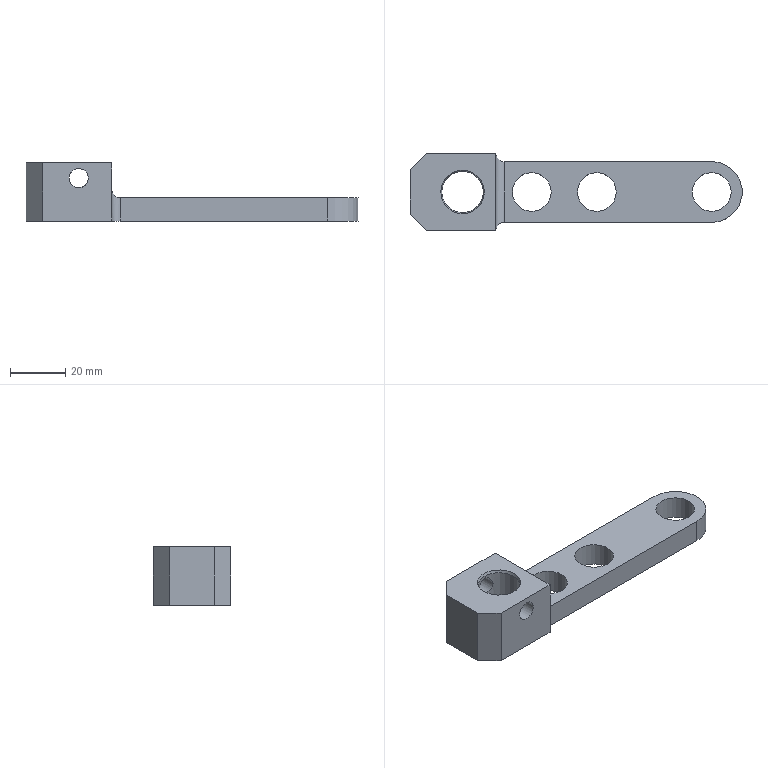Part | NX | 1 solid | 23 faces | box 120 x 28 x 21 mm | volume 25583 mm3 | plane 11 | cylinder 10 | cone 2 | commonest cylinder face diameters 6 x3 14 x3 7 x2 15 x1 22 x1
STEP:
#1=CARTESIAN_POINT('',(26.864,14.,21.));
#2=VERTEX_POINT('',#1);
#3=CARTESIAN_POINT('',(19.,14.,21.));
#4=DIRECTION('',(0.,0.,1.));
#5=DIRECTION('',(1.,0.,0.));
#6=AXIS2_PLACEMENT_3D('',#3,#4,#5);
#7=CIRCLE('',#6,7.864);
#8=EDGE_CURVE('',#2,#2,#7,.F.);
#9=ORIENTED_EDGE('',*,*,#8,.T.);
#10=EDGE_LOOP('',(#9));
#11=FACE_BOUND('',#10,.T.);
#12=CARTESIAN_POINT('',(6.,28.,21.));
#13=VERTEX_POINT('',#12);
#14=CARTESIAN_POINT('',(31.,28.,21.));
#15=VERTEX_POINT('',#14);
#16=CARTESIAN_POINT('',(60.,28.,21.));
#17=DIRECTION('',(1.,0.,0.));
#18=VECTOR('',#17,1000.);
#19=LINE('',#16,#18);
#20=EDGE_CURVE('',#13,#15,#19,.T.);
#21=ORIENTED_EDGE('',*,*,#20,.F.);
#22=CARTESIAN_POINT('',(0.,22.,21.));
#23=VERTEX_POINT('',#22);
#24=CARTESIAN_POINT('',(26.,48.,21.));
#25=DIRECTION('',(0.7071,0.7071,0.));
#26=VECTOR('',#25,1000.);
#27=LINE('',#24,#26);
#28=EDGE_CURVE('',#13,#23,#27,.F.);
#29=ORIENTED_EDGE('',*,*,#28,.T.);
#30=CARTESIAN_POINT('',(0.,6.,21.));
#31=VERTEX_POINT('',#30);
#32=CARTESIAN_POINT('',(0.,14.,21.));
#33=DIRECTION('',(0.,1.,0.));
#34=VECTOR('',#33,1000.);
#35=LINE('',#32,#34);
#36=EDGE_CURVE('',#31,#23,#35,.T.);
#37=ORIENTED_EDGE('',*,*,#36,.F.);
#38=CARTESIAN_POINT('',(6.,0.,21.));
#39=VERTEX_POINT('',#38);
#40=CARTESIAN_POINT('',(26.,-20.,21.));
#41=DIRECTION('',(-0.7071,0.7071,0.));
#42=VECTOR('',#41,1000.);
#43=LINE('',#40,#42);
#44=EDGE_CURVE('',#31,#39,#43,.F.);
#45=ORIENTED_EDGE('',*,*,#44,.T.);
#46=CARTESIAN_POINT('',(31.,0.,21.));
#47=VERTEX_POINT('',#46);
#48=CARTESIAN_POINT('',(60.,0.,21.));
#49=DIRECTION('',(-1.,0.,0.));
#50=VECTOR('',#49,1000.);
#51=LINE('',#48,#50);
#52=EDGE_CURVE('',#47,#39,#51,.T.);
#53=ORIENTED_EDGE('',*,*,#52,.F.);
#54=CARTESIAN_POINT('',(31.,14.,21.));
#55=DIRECTION('',(0.,-1.,0.));
#56=VECTOR('',#55,1000.);
#57=LINE('',#54,#56);
#58=EDGE_CURVE('',#15,#47,#57,.T.);
#59=ORIENTED_EDGE('',*,*,#58,.F.);
#60=EDGE_LOOP('',(#21,#29,#37,#45,#53,#59));
#61=FACE_BOUND('',#60,.T.);
#62=CARTESIAN_POINT('',(60.,14.,21.));
#63=DIRECTION('',(0.,0.,1.));
#64=DIRECTION('',(1.,0.,0.));
#65=AXIS2_PLACEMENT_3D('',#62,#63,#64);
#66=PLANE('',#65);
#67=ADVANCED_FACE('',(#11,#61),#66,.T.);
#68=CARTESIAN_POINT('',(31.,0.,11.5));
#69=VERTEX_POINT('',#68);
#70=CARTESIAN_POINT('',(31.,0.,0.));
#71=DIRECTION('',(0.,0.,-1.));
#72=VECTOR('',#71,1000.);
#73=LINE('',#70,#72);
#74=EDGE_CURVE('',#47,#69,#73,.T.);
#75=ORIENTED_EDGE('',*,*,#74,.T.);
#76=CARTESIAN_POINT('',(31.,28.,11.5));
#77=VERTEX_POINT('',#76);
#78=CARTESIAN_POINT('',(31.,25.,11.5));
#79=DIRECTION('',(0.,1.,0.));
#80=VECTOR('',#79,1000.);
#81=LINE('',#78,#80);
#82=EDGE_CURVE('',#69,#77,#81,.T.);
#83=ORIENTED_EDGE('',*,*,#82,.T.);
#84=CARTESIAN_POINT('',(31.,28.,0.));
#85=DIRECTION('',(0.,0.,1.));
#86=VECTOR('',#85,1000.);
#87=LINE('',#84,#86);
#88=EDGE_CURVE('',#15,#77,#87,.F.);
#89=ORIENTED_EDGE('',*,*,#88,.F.);
#90=ORIENTED_EDGE('',*,*,#58,.T.);
#91=EDGE_LOOP('',(#75,#83,#89,#90));
#92=FACE_BOUND('',#91,.T.);
#93=CARTESIAN_POINT('',(31.,14.,10.5));
#94=DIRECTION('',(-1.,0.,0.));
#95=DIRECTION('',(0.,0.,1.));
#96=AXIS2_PLACEMENT_3D('',#93,#94,#95);
#97=PLANE('',#96);
#98=ADVANCED_FACE('',(#92),#97,.F.);
#99=CARTESIAN_POINT('',(19.008,0.,12.));
#100=VERTEX_POINT('',#99);
#101=CARTESIAN_POINT('',(19.008,0.,15.5));
#102=DIRECTION('',(0.,-1.,0.));
#103=DIRECTION('',(0.,0.,-1.));
#104=AXIS2_PLACEMENT_3D('',#101,#102,#103);
#105=CIRCLE('',#104,3.5);
#106=EDGE_CURVE('',#100,#100,#105,.T.);
#107=ORIENTED_EDGE('',*,*,#106,.F.);
#108=EDGE_LOOP('',(#107));
#109=FACE_BOUND('',#108,.T.);
#110=ORIENTED_EDGE('',*,*,#52,.T.);
#111=CARTESIAN_POINT('',(6.,0.,0.));
#112=VERTEX_POINT('',#111);
#113=CARTESIAN_POINT('',(6.,0.,0.));
#114=DIRECTION('',(0.,0.,-1.));
#115=VECTOR('',#114,1000.);
#116=LINE('',#113,#115);
#117=EDGE_CURVE('',#39,#112,#116,.T.);
#118=ORIENTED_EDGE('',*,*,#117,.T.);
#119=CARTESIAN_POINT('',(31.,0.,0.));
#120=VERTEX_POINT('',#119);
#121=CARTESIAN_POINT('',(60.,0.,0.));
#122=DIRECTION('',(1.,0.,0.));
#123=VECTOR('',#122,1000.);
#124=LINE('',#121,#123);
#125=EDGE_CURVE('',#112,#120,#124,.T.);
#126=ORIENTED_EDGE('',*,*,#125,.T.);
#127=CARTESIAN_POINT('',(31.,0.,0.));
#128=DIRECTION('',(0.,0.,-1.));
#129=VECTOR('',#128,1000.);
#130=LINE('',#127,#129);
#131=EDGE_CURVE('',#69,#120,#130,.T.);
#132=ORIENTED_EDGE('',*,*,#131,.F.);
#133=ORIENTED_EDGE('',*,*,#74,.F.);
#134=EDGE_LOOP('',(#110,#118,#126,#132,#133));
#135=FACE_BOUND('',#134,.T.);
#136=CARTESIAN_POINT('',(60.,0.,0.));
#137=DIRECTION('',(0.,-1.,0.));
#138=DIRECTION('',(0.,0.,-1.));
#139=AXIS2_PLACEMENT_3D('',#136,#137,#138);
#140=PLANE('',#139);
#141=ADVANCED_FACE('',(#109,#135),#140,.T.);
#142=ORIENTED_EDGE('',*,*,#36,.T.);
#143=CARTESIAN_POINT('',(0.,22.,0.));
#144=VERTEX_POINT('',#143);
#145=CARTESIAN_POINT('',(0.,22.,0.));
#146=DIRECTION('',(0.,0.,-1.));
#147=VECTOR('',#146,1000.);
#148=LINE('',#145,#147);
#149=EDGE_CURVE('',#23,#144,#148,.T.);
#150=ORIENTED_EDGE('',*,*,#149,.T.);
#151=CARTESIAN_POINT('',(0.,6.,0.));
#152=VERTEX_POINT('',#151);
#153=CARTESIAN_POINT('',(0.,14.,0.));
#154=DIRECTION('',(0.,-1.,0.));
#155=VECTOR('',#154,1000.);
#156=LINE('',#153,#155);
#157=EDGE_CURVE('',#144,#152,#156,.T.);
#158=ORIENTED_EDGE('',*,*,#157,.T.);
#159=CARTESIAN_POINT('',(0.,6.,0.));
#160=DIRECTION('',(0.,0.,1.));
#161=VECTOR('',#160,1000.);
#162=LINE('',#159,#161);
#163=EDGE_CURVE('',#152,#31,#162,.T.);
#164=ORIENTED_EDGE('',*,*,#163,.T.);
#165=EDGE_LOOP('',(#142,#150,#158,#164));
#166=FACE_BOUND('',#165,.T.);
#167=CARTESIAN_POINT('',(0.,14.,0.));
#168=DIRECTION('',(-1.,0.,0.));
#169=DIRECTION('',(0.,0.,1.));
#170=AXIS2_PLACEMENT_3D('',#167,#168,#169);
#171=PLANE('',#170);
#172=ADVANCED_FACE('',(#166),#171,.T.);
#173=CARTESIAN_POINT('',(19.008,28.,12.));
#174=VERTEX_POINT('',#173);
#175=CARTESIAN_POINT('',(19.008,28.,15.5));
#176=DIRECTION('',(0.,-1.,0.));
#177=DIRECTION('',(0.,0.,-1.));
#178=AXIS2_PLACEMENT_3D('',#175,#176,#177);
#179=CIRCLE('',#178,3.5);
#180=EDGE_CURVE('',#174,#174,#179,.T.);
#181=ORIENTED_EDGE('',*,*,#180,.T.);
#182=EDGE_LOOP('',(#181));
#183=FACE_BOUND('',#182,.T.);
#184=CARTESIAN_POINT('',(31.,28.,0.));
#185=VERTEX_POINT('',#184);
#186=CARTESIAN_POINT('',(6.,28.,0.));
#187=VERTEX_POINT('',#186);
#188=CARTESIAN_POINT('',(60.,28.,0.));
#189=DIRECTION('',(-1.,0.,0.));
#190=VECTOR('',#189,1000.);
#191=LINE('',#188,#190);
#192=EDGE_CURVE('',#185,#187,#191,.T.);
#193=ORIENTED_EDGE('',*,*,#192,.T.);
#194=CARTESIAN_POINT('',(6.,28.,0.));
#195=DIRECTION('',(0.,0.,1.));
#196=VECTOR('',#195,1000.);
#197=LINE('',#194,#196);
#198=EDGE_CURVE('',#187,#13,#197,.T.);
#199=ORIENTED_EDGE('',*,*,#198,.T.);
#200=ORIENTED_EDGE('',*,*,#20,.T.);
#201=ORIENTED_EDGE('',*,*,#88,.T.);
#202=CARTESIAN_POINT('',(31.,28.,0.));
#203=DIRECTION('',(0.,0.,1.));
#204=VECTOR('',#203,1000.);
#205=LINE('',#202,#204);
#206=EDGE_CURVE('',#77,#185,#205,.F.);
#207=ORIENTED_EDGE('',*,*,#206,.T.);
#208=EDGE_LOOP('',(#193,#199,#200,#201,#207));
#209=FACE_BOUND('',#208,.T.);
#210=CARTESIAN_POINT('',(60.,28.,0.));
#211=DIRECTION('',(0.,1.,0.));
#212=DIRECTION('',(0.,0.,1.));
#213=AXIS2_PLACEMENT_3D('',#210,#211,#212);
#214=PLANE('',#213);
#215=ADVANCED_FACE('',(#183,#209),#214,.T.);
#216=CARTESIAN_POINT('',(11.136,14.,0.));
#217=VERTEX_POINT('',#216);
#218=CARTESIAN_POINT('',(19.,14.,0.));
#219=DIRECTION('',(0.,0.,-1.));
#220=DIRECTION('',(-1.,0.,0.));
#221=AXIS2_PLACEMENT_3D('',#218,#219,#220);
#222=CIRCLE('',#221,7.864);
#223=EDGE_CURVE('',#217,#217,#222,.F.);
#224=ORIENTED_EDGE('',*,*,#223,.T.);
#225=EDGE_LOOP('',(#224));
#226=FACE_BOUND('',#225,.T.);
#227=CARTESIAN_POINT('',(102.,14.,0.));
#228=VERTEX_POINT('',#227);
#229=CARTESIAN_POINT('',(109.,14.,0.));
#230=DIRECTION('',(0.,0.,-1.));
#231=DIRECTION('',(-1.,0.,0.));
#232=AXIS2_PLACEMENT_3D('',#229,#230,#231);
#233=CIRCLE('',#232,7.);
#234=EDGE_CURVE('',#228,#228,#233,.T.);
#235=ORIENTED_EDGE('',*,*,#234,.F.);
#236=EDGE_LOOP('',(#235));
#237=FACE_BOUND('',#236,.T.);
#238=CARTESIAN_POINT('',(60.5,14.,0.));
#239=VERTEX_POINT('',#238);
#240=CARTESIAN_POINT('',(67.5,14.,0.));
#241=DIRECTION('',(0.,0.,-1.));
#242=DIRECTION('',(-1.,0.,0.));
#243=AXIS2_PLACEMENT_3D('',#240,#241,#242);
#244=CIRCLE('',#243,7.);
#245=EDGE_CURVE('',#239,#239,#244,.T.);
#246=ORIENTED_EDGE('',*,*,#245,.F.);
#247=EDGE_LOOP('',(#246));
#248=FACE_BOUND('',#247,.T.);
#249=CARTESIAN_POINT('',(37.,14.,0.));
#250=VERTEX_POINT('',#249);
#251=CARTESIAN_POINT('',(44.,14.,0.));
#252=DIRECTION('',(0.,0.,-1.));
#253=DIRECTION('',(-1.,0.,0.));
#254=AXIS2_PLACEMENT_3D('',#251,#252,#253);
#255=CIRCLE('',#254,7.);
#256=EDGE_CURVE('',#250,#250,#255,.T.);
#257=ORIENTED_EDGE('',*,*,#256,.F.);
#258=EDGE_LOOP('',(#257));
#259=FACE_BOUND('',#258,.T.);
#260=ORIENTED_EDGE('',*,*,#157,.F.);
#261=CARTESIAN_POINT('',(26.,48.,0.));
#262=DIRECTION('',(-0.7071,-0.7071,0.));
#263=VECTOR('',#262,1000.);
#264=LINE('',#261,#263);
#265=EDGE_CURVE('',#144,#187,#264,.F.);
#266=ORIENTED_EDGE('',*,*,#265,.T.);
#267=ORIENTED_EDGE('',*,*,#192,.F.);
#268=CARTESIAN_POINT('',(34.,25.,0.));
#269=VERTEX_POINT('',#268);
#270=CARTESIAN_POINT('',(34.,28.,0.));
#271=DIRECTION('',(0.,0.,-1.));
#272=DIRECTION('',(-1.,0.,0.));
#273=AXIS2_PLACEMENT_3D('',#270,#271,#272);
#274=CIRCLE('',#273,3.);
#275=EDGE_CURVE('',#185,#269,#274,.F.);
#276=ORIENTED_EDGE('',*,*,#275,.T.);
#277=CARTESIAN_POINT('',(109.,25.,0.));
#278=VERTEX_POINT('',#277);
#279=CARTESIAN_POINT('',(60.,25.,0.));
#280=DIRECTION('',(-1.,0.,0.));
#281=VECTOR('',#280,1000.);
#282=LINE('',#279,#281);
#283=EDGE_CURVE('',#278,#269,#282,.T.);
#284=ORIENTED_EDGE('',*,*,#283,.F.);
#285=CARTESIAN_POINT('',(109.,3.,0.));
#286=VERTEX_POINT('',#285);
#287=CARTESIAN_POINT('',(109.,14.,0.));
#288=DIRECTION('',(0.,0.,-1.));
#289=DIRECTION('',(-1.,0.,0.));
#290=AXIS2_PLACEMENT_3D('',#287,#288,#289);
#291=CIRCLE('',#290,11.);
#292=EDGE_CURVE('',#278,#286,#291,.T.);
#293=ORIENTED_EDGE('',*,*,#292,.T.);
#294=CARTESIAN_POINT('',(34.,3.,0.));
#295=VERTEX_POINT('',#294);
#296=CARTESIAN_POINT('',(60.,3.,0.));
#297=DIRECTION('',(1.,0.,0.));
#298=VECTOR('',#297,1000.);
#299=LINE('',#296,#298);
#300=EDGE_CURVE('',#295,#286,#299,.T.);
#301=ORIENTED_EDGE('',*,*,#300,.F.);
#302=CARTESIAN_POINT('',(34.,0.,0.));
#303=DIRECTION('',(0.,0.,-1.));
#304=DIRECTION('',(-1.,0.,0.));
#305=AXIS2_PLACEMENT_3D('',#302,#303,#304);
#306=CIRCLE('',#305,3.);
#307=EDGE_CURVE('',#295,#120,#306,.F.);
#308=ORIENTED_EDGE('',*,*,#307,.T.);
#309=ORIENTED_EDGE('',*,*,#125,.F.);
#310=CARTESIAN_POINT('',(26.,-20.,0.));
#311=DIRECTION('',(0.7071,-0.7071,0.));
#312=VECTOR('',#311,1000.);
#313=LINE('',#310,#312);
#314=EDGE_CURVE('',#112,#152,#313,.F.);
#315=ORIENTED_EDGE('',*,*,#314,.T.);
#316=EDGE_LOOP('',(#260,#266,#267,#276,#284,#293,#301,#308,#309,#315));
#317=FACE_BOUND('',#316,.T.);
#318=CARTESIAN_POINT('',(60.,14.,0.));
#319=DIRECTION('',(0.,0.,-1.));
#320=DIRECTION('',(-1.,0.,0.));
#321=AXIS2_PLACEMENT_3D('',#318,#319,#320);
#322=PLANE('',#321);
#323=ADVANCED_FACE('',(#226,#237,#248,#259,#317),#322,.T.);
#324=ORIENTED_EDGE('',*,*,#265,.F.);
#325=ORIENTED_EDGE('',*,*,#149,.F.);
#326=ORIENTED_EDGE('',*,*,#28,.F.);
#327=ORIENTED_EDGE('',*,*,#198,.F.);
#328=EDGE_LOOP('',(#324,#325,#326,#327));
#329=FACE_BOUND('',#328,.T.);
#330=CARTESIAN_POINT('',(6.,28.,0.));
#331=DIRECTION('',(0.7071,-0.7071,0.));
#332=DIRECTION('',(0.,0.,1.));
#333=AXIS2_PLACEMENT_3D('',#330,#331,#332);
#334=PLANE('',#333);
#335=ADVANCED_FACE('',(#329),#334,.F.);
#336=ORIENTED_EDGE('',*,*,#314,.F.);
#337=ORIENTED_EDGE('',*,*,#117,.F.);
#338=ORIENTED_EDGE('',*,*,#44,.F.);
#339=ORIENTED_EDGE('',*,*,#163,.F.);
#340=EDGE_LOOP('',(#336,#337,#338,#339));
#341=FACE_BOUND('',#340,.T.);
#342=CARTESIAN_POINT('',(0.,6.,0.));
#343=DIRECTION('',(0.7071,0.7071,0.));
#344=DIRECTION('',(0.,0.,1.));
#345=AXIS2_PLACEMENT_3D('',#342,#343,#344);
#346=PLANE('',#345);
#347=ADVANCED_FACE('',(#341),#346,.F.);
#348=ORIENTED_EDGE('',*,*,#283,.T.);
#349=CARTESIAN_POINT('',(34.,25.,8.5));
#350=VERTEX_POINT('',#349);
#351=CARTESIAN_POINT('',(34.,25.,0.));
#352=DIRECTION('',(0.,0.,-1.));
#353=VECTOR('',#352,1000.);
#354=LINE('',#351,#353);
#355=EDGE_CURVE('',#269,#350,#354,.F.);
#356=ORIENTED_EDGE('',*,*,#355,.T.);
#357=CARTESIAN_POINT('',(109.,25.,8.5));
#358=VERTEX_POINT('',#357);
#359=CARTESIAN_POINT('',(75.5,25.,8.5));
#360=DIRECTION('',(1.,0.,0.));
#361=VECTOR('',#360,1000.);
#362=LINE('',#359,#361);
#363=EDGE_CURVE('',#350,#358,#362,.T.);
#364=ORIENTED_EDGE('',*,*,#363,.T.);
#365=CARTESIAN_POINT('',(109.,25.,0.));
#366=DIRECTION('',(0.,0.,1.));
#367=VECTOR('',#366,1000.);
#368=LINE('',#365,#367);
#369=EDGE_CURVE('',#358,#278,#368,.F.);
#370=ORIENTED_EDGE('',*,*,#369,.T.);
#371=EDGE_LOOP('',(#348,#356,#364,#370));
#372=FACE_BOUND('',#371,.T.);
#373=CARTESIAN_POINT('',(60.,25.,0.));
#374=DIRECTION('',(0.,1.,0.));
#375=DIRECTION('',(0.,0.,1.));
#376=AXIS2_PLACEMENT_3D('',#373,#374,#375);
#377=PLANE('',#376);
#378=ADVANCED_FACE('',(#372),#377,.T.);
#379=CARTESIAN_POINT('',(34.,3.,8.5));
#380=VERTEX_POINT('',#379);
#381=CARTESIAN_POINT('',(109.,3.,8.5));
#382=VERTEX_POINT('',#381);
#383=CARTESIAN_POINT('',(60.,3.,8.5));
#384=DIRECTION('',(1.,0.,0.));
#385=VECTOR('',#384,1000.);
#386=LINE('',#383,#385);
#387=EDGE_CURVE('',#380,#382,#386,.T.);
#388=ORIENTED_EDGE('',*,*,#387,.F.);
#389=CARTESIAN_POINT('',(34.,3.,0.));
#390=DIRECTION('',(0.,0.,1.));
#391=VECTOR('',#390,1000.);
#392=LINE('',#389,#391);
#393=EDGE_CURVE('',#380,#295,#392,.F.);
#394=ORIENTED_EDGE('',*,*,#393,.T.);
#395=ORIENTED_EDGE('',*,*,#300,.T.);
#396=CARTESIAN_POINT('',(109.,3.,0.));
#397=DIRECTION('',(0.,0.,1.));
#398=VECTOR('',#397,1000.);
#399=LINE('',#396,#398);
#400=EDGE_CURVE('',#286,#382,#399,.T.);
#401=ORIENTED_EDGE('',*,*,#400,.T.);
#402=EDGE_LOOP('',(#388,#394,#395,#401));
#403=FACE_BOUND('',#402,.T.);
#404=CARTESIAN_POINT('',(60.,3.,0.));
#405=DIRECTION('',(0.,-1.,0.));
#406=DIRECTION('',(0.,0.,-1.));
#407=AXIS2_PLACEMENT_3D('',#404,#405,#406);
#408=PLANE('',#407);
#409=ADVANCED_FACE('',(#403),#408,.T.);
#410=CARTESIAN_POINT('',(102.,14.,8.5));
#411=VERTEX_POINT('',#410);
#412=CARTESIAN_POINT('',(109.,14.,8.5));
#413=DIRECTION('',(0.,0.,-1.));
#414=DIRECTION('',(-1.,0.,0.));
#415=AXIS2_PLACEMENT_3D('',#412,#413,#414);
#416=CIRCLE('',#415,7.);
#417=EDGE_CURVE('',#411,#411,#416,.T.);
#418=ORIENTED_EDGE('',*,*,#417,.T.);
#419=EDGE_LOOP('',(#418));
#420=FACE_BOUND('',#419,.T.);
#421=CARTESIAN_POINT('',(60.5,14.,8.5));
#422=VERTEX_POINT('',#421);
#423=CARTESIAN_POINT('',(67.5,14.,8.5));
#424=DIRECTION('',(0.,0.,-1.));
#425=DIRECTION('',(-1.,0.,0.));
#426=AXIS2_PLACEMENT_3D('',#423,#424,#425);
#427=CIRCLE('',#426,7.);
#428=EDGE_CURVE('',#422,#422,#427,.T.);
#429=ORIENTED_EDGE('',*,*,#428,.T.);
#430=EDGE_LOOP('',(#429));
#431=FACE_BOUND('',#430,.T.);
#432=CARTESIAN_POINT('',(37.,14.,8.5));
#433=VERTEX_POINT('',#432);
#434=CARTESIAN_POINT('',(44.,14.,8.5));
#435=DIRECTION('',(0.,0.,-1.));
#436=DIRECTION('',(-1.,0.,0.));
#437=AXIS2_PLACEMENT_3D('',#434,#435,#436);
#438=CIRCLE('',#437,7.);
#439=EDGE_CURVE('',#433,#433,#438,.T.);
#440=ORIENTED_EDGE('',*,*,#439,.T.);
#441=EDGE_LOOP('',(#440));
#442=FACE_BOUND('',#441,.T.);
#443=ORIENTED_EDGE('',*,*,#363,.F.);
#444=CARTESIAN_POINT('',(34.,3.,8.5));
#445=DIRECTION('',(0.,1.,0.));
#446=VECTOR('',#445,1000.);
#447=LINE('',#444,#446);
#448=EDGE_CURVE('',#350,#380,#447,.F.);
#449=ORIENTED_EDGE('',*,*,#448,.T.);
#450=ORIENTED_EDGE('',*,*,#387,.T.);
#451=CARTESIAN_POINT('',(109.,14.,8.5));
#452=DIRECTION('',(0.,0.,-1.));
#453=DIRECTION('',(-1.,0.,0.));
#454=AXIS2_PLACEMENT_3D('',#451,#452,#453);
#455=CIRCLE('',#454,11.);
#456=EDGE_CURVE('',#382,#358,#455,.F.);
#457=ORIENTED_EDGE('',*,*,#456,.T.);
#458=EDGE_LOOP('',(#443,#449,#450,#457));
#459=FACE_BOUND('',#458,.T.);
#460=CARTESIAN_POINT('',(75.5,14.,8.5));
#461=DIRECTION('',(0.,0.,-1.));
#462=DIRECTION('',(-1.,0.,0.));
#463=AXIS2_PLACEMENT_3D('',#460,#461,#462);
#464=PLANE('',#463);
#465=ADVANCED_FACE('',(#420,#431,#442,#459),#464,.F.);
#466=ORIENTED_EDGE('',*,*,#456,.F.);
#467=ORIENTED_EDGE('',*,*,#400,.F.);
#468=ORIENTED_EDGE('',*,*,#292,.F.);
#469=ORIENTED_EDGE('',*,*,#369,.F.);
#470=EDGE_LOOP('',(#466,#467,#468,#469));
#471=FACE_BOUND('',#470,.T.);
#472=CARTESIAN_POINT('',(109.,14.,0.));
#473=DIRECTION('',(0.,0.,1.));
#474=DIRECTION('',(1.,0.,0.));
#475=AXIS2_PLACEMENT_3D('',#472,#473,#474);
#476=CYLINDRICAL_SURFACE('',#475,11.);
#477=ADVANCED_FACE('',(#471),#476,.T.);
#478=ORIENTED_EDGE('',*,*,#307,.F.);
#479=ORIENTED_EDGE('',*,*,#393,.F.);
#480=CARTESIAN_POINT('',(34.,0.,11.5));
#481=DIRECTION('',(0.,-0.7071,-0.7071));
#482=DIRECTION('',(0.,-0.7071,0.7071));
#483=AXIS2_PLACEMENT_3D('',#480,#481,#482);
#484=ELLIPSE('',#483,4.243,3.);
#485=EDGE_CURVE('',#69,#380,#484,.T.);
#486=ORIENTED_EDGE('',*,*,#485,.F.);
#487=ORIENTED_EDGE('',*,*,#131,.T.);
#488=EDGE_LOOP('',(#478,#479,#486,#487));
#489=FACE_BOUND('',#488,.T.);
#490=CARTESIAN_POINT('',(34.,0.,10.5));
#491=DIRECTION('',(0.,0.,1.));
#492=DIRECTION('',(1.,0.,0.));
#493=AXIS2_PLACEMENT_3D('',#490,#491,#492);
#494=CYLINDRICAL_SURFACE('',#493,3.);
#495=ADVANCED_FACE('',(#489),#494,.F.);
#496=ORIENTED_EDGE('',*,*,#485,.T.);
#497=ORIENTED_EDGE('',*,*,#448,.F.);
#498=CARTESIAN_POINT('',(34.,28.,11.5));
#499=DIRECTION('',(0.,0.7071,-0.7071));
#500=DIRECTION('',(0.,-0.7071,-0.7071));
#501=AXIS2_PLACEMENT_3D('',#498,#499,#500);
#502=ELLIPSE('',#501,4.243,3.);
#503=EDGE_CURVE('',#77,#350,#502,.F.);
#504=ORIENTED_EDGE('',*,*,#503,.F.);
#505=ORIENTED_EDGE('',*,*,#82,.F.);
#506=EDGE_LOOP('',(#496,#497,#504,#505));
#507=FACE_BOUND('',#506,.T.);
#508=CARTESIAN_POINT('',(34.,14.,11.5));
#509=DIRECTION('',(0.,-1.,0.));
#510=DIRECTION('',(0.,0.,-1.));
#511=AXIS2_PLACEMENT_3D('',#508,#509,#510);
#512=CYLINDRICAL_SURFACE('',#511,3.);
#513=ADVANCED_FACE('',(#507),#512,.F.);
#514=ORIENTED_EDGE('',*,*,#275,.F.);
#515=ORIENTED_EDGE('',*,*,#206,.F.);
#516=ORIENTED_EDGE('',*,*,#503,.T.);
#517=ORIENTED_EDGE('',*,*,#355,.F.);
#518=EDGE_LOOP('',(#514,#515,#516,#517));
#519=FACE_BOUND('',#518,.T.);
#520=CARTESIAN_POINT('',(34.,28.,10.5));
#521=DIRECTION('',(0.,0.,-1.));
#522=DIRECTION('',(-1.,0.,0.));
#523=AXIS2_PLACEMENT_3D('',#520,#521,#522);
#524=CYLINDRICAL_SURFACE('',#523,3.);
#525=ADVANCED_FACE('',(#519),#524,.F.);
#526=ORIENTED_EDGE('',*,*,#256,.T.);
#527=EDGE_LOOP('',(#526));
#528=FACE_BOUND('',#527,.T.);
#529=ORIENTED_EDGE('',*,*,#439,.F.);
#530=EDGE_LOOP('',(#529));
#531=FACE_BOUND('',#530,.T.);
#532=CARTESIAN_POINT('',(44.,14.,12.5));
#533=DIRECTION('',(0.,0.,-1.));
#534=DIRECTION('',(-1.,0.,0.));
#535=AXIS2_PLACEMENT_3D('',#532,#533,#534);
#536=CYLINDRICAL_SURFACE('',#535,7.);
#537=ADVANCED_FACE('',(#528,#531),#536,.F.);
#538=ORIENTED_EDGE('',*,*,#245,.T.);
#539=EDGE_LOOP('',(#538));
#540=FACE_BOUND('',#539,.T.);
#541=ORIENTED_EDGE('',*,*,#428,.F.);
#542=EDGE_LOOP('',(#541));
#543=FACE_BOUND('',#542,.T.);
#544=CARTESIAN_POINT('',(67.5,14.,12.5));
#545=DIRECTION('',(0.,0.,-1.));
#546=DIRECTION('',(-1.,0.,0.));
#547=AXIS2_PLACEMENT_3D('',#544,#545,#546);
#548=CYLINDRICAL_SURFACE('',#547,7.);
#549=ADVANCED_FACE('',(#540,#543),#548,.F.);
#550=ORIENTED_EDGE('',*,*,#234,.T.);
#551=EDGE_LOOP('',(#550));
#552=FACE_BOUND('',#551,.T.);
#553=ORIENTED_EDGE('',*,*,#417,.F.);
#554=EDGE_LOOP('',(#553));
#555=FACE_BOUND('',#554,.T.);
#556=CARTESIAN_POINT('',(109.,14.,12.5));
#557=DIRECTION('',(0.,0.,-1.));
#558=DIRECTION('',(-1.,0.,0.));
#559=AXIS2_PLACEMENT_3D('',#556,#557,#558);
#560=CYLINDRICAL_SURFACE('',#559,7.);
#561=ADVANCED_FACE('',(#552,#555),#560,.F.);
#562=CARTESIAN_POINT('',(11.5,14.,1.));
#563=VERTEX_POINT('',#562);
#564=CARTESIAN_POINT('',(19.,14.,1.));
#565=DIRECTION('',(0.,0.,-1.));
#566=DIRECTION('',(-1.,0.,0.));
#567=AXIS2_PLACEMENT_3D('',#564,#565,#566);
#568=CIRCLE('',#567,7.5);
#569=EDGE_CURVE('',#563,#563,#568,.T.);
#570=ORIENTED_EDGE('',*,*,#569,.T.);
#571=EDGE_LOOP('',(#570));
#572=FACE_BOUND('',#571,.T.);
#573=CARTESIAN_POINT('',(26.5,14.,20.));
#574=VERTEX_POINT('',#573);
#575=CARTESIAN_POINT('',(19.,14.,20.));
#576=DIRECTION('',(0.,0.,1.));
#577=DIRECTION('',(1.,0.,0.));
#578=AXIS2_PLACEMENT_3D('',#575,#576,#577);
#579=CIRCLE('',#578,7.5);
#580=EDGE_CURVE('',#574,#574,#579,.T.);
#581=ORIENTED_EDGE('',*,*,#580,.T.);
#582=EDGE_LOOP('',(#581));
#583=FACE_BOUND('',#582,.T.);
#584=CARTESIAN_POINT('',(19.008,21.5,12.));
#585=VERTEX_POINT('',#584);
#586=CARTESIAN_POINT('',(21.755,21.089,12.76));
#587=CARTESIAN_POINT('',(19.007,21.704,11.619));
#588=CARTESIAN_POINT('',(16.263,21.095,12.762));
#589=CARTESIAN_POINT('',(15.13,20.409,15.491));
#590=CARTESIAN_POINT('',(16.263,21.094,18.241));
#591=CARTESIAN_POINT('',(18.999,21.704,19.38));
#592=CARTESIAN_POINT('',(21.753,21.09,18.241));
#593=CARTESIAN_POINT('',(22.885,20.399,15.508));
#594=CARTESIAN_POINT('',(21.755,21.089,12.76));
#595=CARTESIAN_POINT('',(19.007,21.704,11.619));
#596=CARTESIAN_POINT('',(16.263,21.095,12.762));
#597=B_SPLINE_CURVE_WITH_KNOTS('',3,(#586,#587,#588,#589,#590,#591,#592,#593,#594,#595,#596),.UNSPECIFIED.,.T.,.F.,(1,1,1,1,1,1,1,1,1,1,1,1,1,1,1),(-0.008324,-0.005549,-0.002775,0.,0.002775,0.005549,0.008324,0.0111,0.01387,0.01665,0.01942,0.0222,0.02497,0.02775,0.03052),.UNSPECIFIED.);
#598=EDGE_CURVE('',#585,#585,#597,.T.);
#599=ORIENTED_EDGE('',*,*,#598,.T.);
#600=EDGE_LOOP('',(#599));
#601=FACE_BOUND('',#600,.T.);
#602=CARTESIAN_POINT('',(19.008,6.5,12.));
#603=VERTEX_POINT('',#602);
#604=CARTESIAN_POINT('',(16.259,6.906,12.76));
#605=CARTESIAN_POINT('',(19.009,6.296,11.619));
#606=CARTESIAN_POINT('',(21.751,6.91,12.762));
#607=CARTESIAN_POINT('',(22.885,7.601,15.489));
#608=CARTESIAN_POINT('',(21.754,6.912,18.239));
#609=CARTESIAN_POINT('',(19.02,6.296,19.38));
#610=CARTESIAN_POINT('',(16.264,6.903,18.242));
#611=CARTESIAN_POINT('',(15.131,7.592,15.51));
#612=CARTESIAN_POINT('',(16.259,6.906,12.76));
#613=CARTESIAN_POINT('',(19.009,6.296,11.619));
#614=CARTESIAN_POINT('',(21.751,6.91,12.762));
#615=B_SPLINE_CURVE_WITH_KNOTS('',3,(#604,#605,#606,#607,#608,#609,#610,#611,#612,#613,#614),.UNSPECIFIED.,.T.,.F.,(1,1,1,1,1,1,1,1,1,1,1,1,1,1,1),(-0.008324,-0.005549,-0.002775,0.,0.002775,0.005549,0.008324,0.0111,0.01387,0.01665,0.01942,0.0222,0.02497,0.02775,0.03052),.UNSPECIFIED.);
#616=EDGE_CURVE('',#603,#603,#615,.T.);
#617=ORIENTED_EDGE('',*,*,#616,.T.);
#618=EDGE_LOOP('',(#617));
#619=FACE_BOUND('',#618,.T.);
#620=CARTESIAN_POINT('',(19.,14.,12.5));
#621=DIRECTION('',(0.,0.,-1.));
#622=DIRECTION('',(-1.,0.,0.));
#623=AXIS2_PLACEMENT_3D('',#620,#621,#622);
#624=CYLINDRICAL_SURFACE('',#623,7.5);
#625=ADVANCED_FACE('',(#572,#583,#601,#619),#624,.F.);
#626=ORIENTED_EDGE('',*,*,#106,.T.);
#627=EDGE_LOOP('',(#626));
#628=FACE_BOUND('',#627,.T.);
#629=ORIENTED_EDGE('',*,*,#616,.F.);
#630=EDGE_LOOP('',(#629));
#631=FACE_BOUND('',#630,.T.);
#632=CARTESIAN_POINT('',(19.008,28.,15.5));
#633=DIRECTION('',(0.,-1.,0.));
#634=DIRECTION('',(0.,0.,-1.));
#635=AXIS2_PLACEMENT_3D('',#632,#633,#634);
#636=CYLINDRICAL_SURFACE('',#635,3.5);
#637=ADVANCED_FACE('',(#628,#631),#636,.F.);
#638=ORIENTED_EDGE('',*,*,#180,.F.);
#639=EDGE_LOOP('',(#638));
#640=FACE_BOUND('',#639,.T.);
#641=ORIENTED_EDGE('',*,*,#598,.F.);
#642=EDGE_LOOP('',(#641));
#643=FACE_BOUND('',#642,.T.);
#644=CARTESIAN_POINT('',(19.008,28.,15.5));
#645=DIRECTION('',(0.,-1.,0.));
#646=DIRECTION('',(0.,0.,-1.));
#647=AXIS2_PLACEMENT_3D('',#644,#645,#646);
#648=CYLINDRICAL_SURFACE('',#647,3.5);
#649=ADVANCED_FACE('',(#640,#643),#648,.F.);
#650=ORIENTED_EDGE('',*,*,#223,.F.);
#651=EDGE_LOOP('',(#650));
#652=FACE_BOUND('',#651,.T.);
#653=ORIENTED_EDGE('',*,*,#569,.F.);
#654=EDGE_LOOP('',(#653));
#655=FACE_BOUND('',#654,.T.);
#656=CARTESIAN_POINT('',(19.,14.,1.));
#657=DIRECTION('',(0.,0.,-1.));
#658=DIRECTION('',(-1.,0.,0.));
#659=AXIS2_PLACEMENT_3D('',#656,#657,#658);
#660=CONICAL_SURFACE('',#659,7.5,0.3491);
#661=ADVANCED_FACE('',(#652,#655),#660,.F.);
#662=ORIENTED_EDGE('',*,*,#8,.F.);
#663=EDGE_LOOP('',(#662));
#664=FACE_BOUND('',#663,.T.);
#665=ORIENTED_EDGE('',*,*,#580,.F.);
#666=EDGE_LOOP('',(#665));
#667=FACE_BOUND('',#666,.T.);
#668=CARTESIAN_POINT('',(19.,14.,20.));
#669=DIRECTION('',(0.,0.,1.));
#670=DIRECTION('',(1.,0.,0.));
#671=AXIS2_PLACEMENT_3D('',#668,#669,#670);
#672=CONICAL_SURFACE('',#671,7.5,0.3491);
#673=ADVANCED_FACE('',(#664,#667),#672,.F.);
#674=CLOSED_SHELL('',(#67,#98,#141,#172,#215,#323,#335,#347,#378,#409,#465,#477,#495,#513,#525,#537,#549,#561,#625,#637,#649,#661,#673));
#675=MANIFOLD_SOLID_BREP('',#674);
#676=(LENGTH_UNIT()NAMED_UNIT(*)SI_UNIT(.MILLI.,.METRE.));
#677=UNCERTAINTY_MEASURE_WITH_UNIT(LENGTH_MEASURE(0.0508),#676,'','');
#678=(NAMED_UNIT(*)PLANE_ANGLE_UNIT()SI_UNIT($,.RADIAN.));
#679=(NAMED_UNIT(*)SI_UNIT($,.STERADIAN.)SOLID_ANGLE_UNIT());
#680=(GEOMETRIC_REPRESENTATION_CONTEXT(3)GLOBAL_UNCERTAINTY_ASSIGNED_CONTEXT((#677))GLOBAL_UNIT_ASSIGNED_CONTEXT((#676,#678,#679))REPRESENTATION_CONTEXT('',''));
#681=ADVANCED_BREP_SHAPE_REPRESENTATION('',(#675),#680);